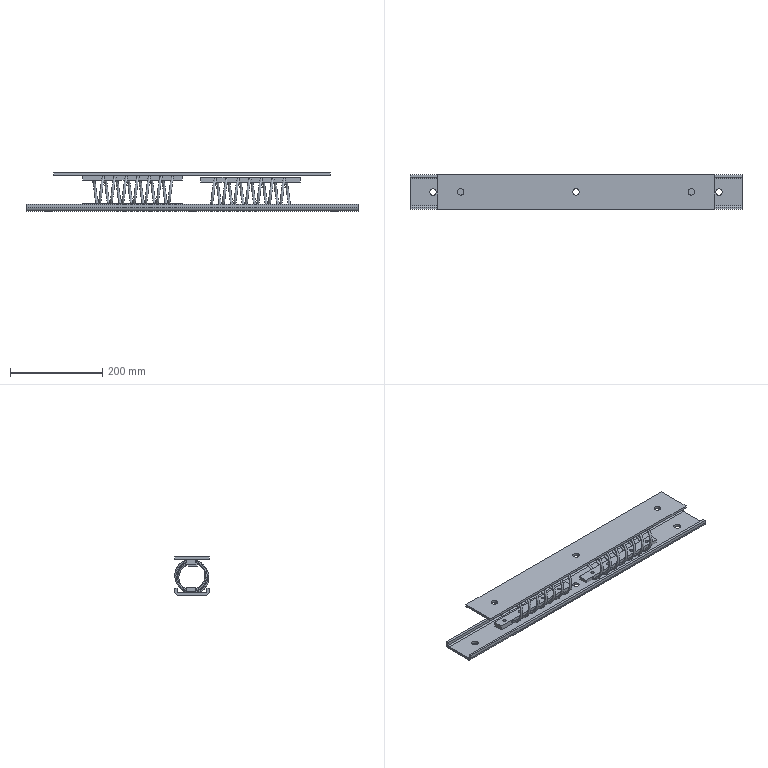Part | SolidWorks | 4 solids | 144 faces | box 720 x 75 x 82.954 mm | volume 767649 mm3 | spline 56 | cylinder 48 | plane 40 | commonest cylinder face diameters 6.8 x32 14 x12 6 x2 16 x2